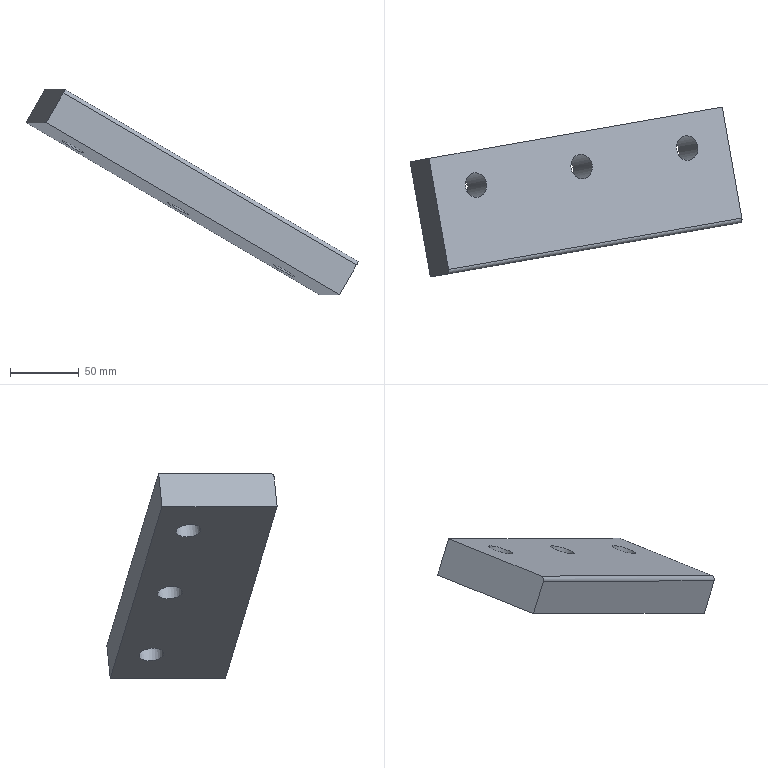Part | NX | features solid 2 | 1 solid | 10 faces | box 241.333 x 123.736 x 149.249 mm | volume 573142 mm3 | plane 6 | cylinder 4 | commonest cylinder face diameters 18 x3 6 x1
STEP:
#1=CARTESIAN_POINT('',(990.848,746.001,-183.512));
#2=VERTEX_POINT('',#1);
#3=CARTESIAN_POINT('',(777.631,708.405,-58.512));
#4=VERTEX_POINT('',#3);
#5=CARTESIAN_POINT('',(990.848,746.001,-183.512));
#6=DIRECTION('',(-0.8529,-0.1504,0.5));
#7=VECTOR('',#6,1000.);
#8=LINE('',#5,#7);
#9=EDGE_CURVE('',#2,#4,#8,.T.);
#10=ORIENTED_EDGE('',*,*,#9,.T.);
#11=CARTESIAN_POINT('',(791.418,710.836,-34.264));
#12=VERTEX_POINT('',#11);
#13=CARTESIAN_POINT('',(791.418,710.836,-34.264));
#14=DIRECTION('',(-0.4924,-0.08682,-0.866));
#15=VECTOR('',#14,1000.);
#16=LINE('',#13,#15);
#17=EDGE_CURVE('',#12,#4,#16,.T.);
#18=ORIENTED_EDGE('',*,*,#17,.F.);
#19=CARTESIAN_POINT('',(1004.635,748.432,-159.264));
#20=VERTEX_POINT('',#19);
#21=CARTESIAN_POINT('',(1004.635,748.432,-159.264));
#22=DIRECTION('',(-0.8529,-0.1504,0.5));
#23=VECTOR('',#22,1000.);
#24=LINE('',#21,#23);
#25=EDGE_CURVE('',#20,#12,#24,.T.);
#26=ORIENTED_EDGE('',*,*,#25,.F.);
#27=CARTESIAN_POINT('',(1004.635,748.432,-159.264));
#28=DIRECTION('',(-0.4924,-0.08682,-0.866));
#29=VECTOR('',#28,1000.);
#30=LINE('',#27,#29);
#31=EDGE_CURVE('',#20,#2,#30,.T.);
#32=ORIENTED_EDGE('',*,*,#31,.T.);
#33=EDGE_LOOP('',(#10,#18,#26,#32));
#34=FACE_BOUND('',#33,.T.);
#35=CARTESIAN_POINT('',(1004.635,748.432,-159.264));
#36=DIRECTION('',(-0.1736,0.9848,0.));
#37=DIRECTION('',(0.8529,0.1504,-0.5));
#38=AXIS2_PLACEMENT_3D('',#35,#36,#37);
#39=PLANE('',#38);
#40=ADVANCED_FACE('',(#34),#39,.T.);
#41=CARTESIAN_POINT('',(805.657,630.082,-34.264));
#42=VERTEX_POINT('',#41);
#43=CARTESIAN_POINT('',(792.807,702.957,-34.264));
#44=DIRECTION('',(0.1736,-0.9848,0.));
#45=VECTOR('',#44,1000.);
#46=LINE('',#43,#45);
#47=EDGE_CURVE('',#12,#42,#46,.T.);
#48=ORIENTED_EDGE('',*,*,#47,.F.);
#49=ORIENTED_EDGE('',*,*,#17,.T.);
#50=CARTESIAN_POINT('',(792.391,624.696,-58.512));
#51=VERTEX_POINT('',#50);
#52=CARTESIAN_POINT('',(779.02,700.526,-58.512));
#53=DIRECTION('',(0.1736,-0.9848,0.));
#54=VECTOR('',#53,1000.);
#55=LINE('',#52,#54);
#56=EDGE_CURVE('',#4,#51,#55,.T.);
#57=ORIENTED_EDGE('',*,*,#56,.T.);
#58=CARTESIAN_POINT('',(804.701,626.867,-36.862));
#59=VERTEX_POINT('',#58);
#60=CARTESIAN_POINT('',(806.178,627.127,-34.264));
#61=DIRECTION('',(-0.4924,-0.08682,-0.866));
#62=VECTOR('',#61,1000.);
#63=LINE('',#60,#62);
#64=EDGE_CURVE('',#59,#51,#63,.T.);
#65=ORIENTED_EDGE('',*,*,#64,.F.);
#66=CARTESIAN_POINT('',(804.18,629.821,-36.862));
#67=DIRECTION('',(0.8529,0.1504,-0.5));
#68=DIRECTION('',(0.4924,0.08682,0.866));
#69=AXIS2_PLACEMENT_3D('',#66,#67,#68);
#70=CIRCLE('',#69,3.);
#71=EDGE_CURVE('',#42,#59,#70,.T.);
#72=ORIENTED_EDGE('',*,*,#71,.F.);
#73=EDGE_LOOP('',(#48,#49,#57,#65,#72));
#74=FACE_BOUND('',#73,.T.);
#75=CARTESIAN_POINT('',(792.807,702.957,-34.264));
#76=DIRECTION('',(-0.8529,-0.1504,0.5));
#77=DIRECTION('',(0.4924,0.08682,0.866));
#78=AXIS2_PLACEMENT_3D('',#75,#76,#77);
#79=PLANE('',#78);
#80=ADVANCED_FACE('',(#74),#79,.T.);
#81=ORIENTED_EDGE('',*,*,#64,.T.);
#82=CARTESIAN_POINT('',(1005.608,662.292,-183.512));
#83=VERTEX_POINT('',#82);
#84=CARTESIAN_POINT('',(1005.608,662.292,-183.512));
#85=DIRECTION('',(0.8529,0.1504,-0.5));
#86=VECTOR('',#85,1000.);
#87=LINE('',#84,#86);
#88=EDGE_CURVE('',#51,#83,#87,.T.);
#89=ORIENTED_EDGE('',*,*,#88,.T.);
#90=CARTESIAN_POINT('',(1017.918,664.463,-161.862));
#91=VERTEX_POINT('',#90);
#92=CARTESIAN_POINT('',(1019.396,664.723,-159.264));
#93=DIRECTION('',(-0.4924,-0.08682,-0.866));
#94=VECTOR('',#93,1000.);
#95=LINE('',#92,#94);
#96=EDGE_CURVE('',#91,#83,#95,.T.);
#97=ORIENTED_EDGE('',*,*,#96,.F.);
#98=CARTESIAN_POINT('',(804.701,626.867,-36.862));
#99=DIRECTION('',(0.8529,0.1504,-0.5));
#100=VECTOR('',#99,1000.);
#101=LINE('',#98,#100);
#102=EDGE_CURVE('',#59,#91,#101,.T.);
#103=ORIENTED_EDGE('',*,*,#102,.F.);
#104=EDGE_LOOP('',(#81,#89,#97,#103));
#105=FACE_BOUND('',#104,.T.);
#106=CARTESIAN_POINT('',(806.178,627.127,-34.264));
#107=DIRECTION('',(0.1736,-0.9848,0.));
#108=DIRECTION('',(0.4924,0.08682,0.866));
#109=AXIS2_PLACEMENT_3D('',#106,#107,#108);
#110=PLANE('',#109);
#111=ADVANCED_FACE('',(#105),#110,.T.);
#112=ORIENTED_EDGE('',*,*,#96,.T.);
#113=CARTESIAN_POINT('',(992.237,738.122,-183.512));
#114=DIRECTION('',(-0.1736,0.9848,0.));
#115=VECTOR('',#114,1000.);
#116=LINE('',#113,#115);
#117=EDGE_CURVE('',#83,#2,#116,.T.);
#118=ORIENTED_EDGE('',*,*,#117,.T.);
#119=ORIENTED_EDGE('',*,*,#31,.F.);
#120=CARTESIAN_POINT('',(1018.875,667.677,-159.264));
#121=VERTEX_POINT('',#120);
#122=CARTESIAN_POINT('',(1018.527,669.647,-159.264));
#123=DIRECTION('',(-0.1736,0.9848,0.));
#124=VECTOR('',#123,1000.);
#125=LINE('',#122,#124);
#126=EDGE_CURVE('',#121,#20,#125,.T.);
#127=ORIENTED_EDGE('',*,*,#126,.F.);
#128=CARTESIAN_POINT('',(1017.397,667.417,-161.862));
#129=DIRECTION('',(-0.8529,-0.1504,0.5));
#130=DIRECTION('',(0.1736,-0.9848,0.));
#131=AXIS2_PLACEMENT_3D('',#128,#129,#130);
#132=CIRCLE('',#131,3.);
#133=EDGE_CURVE('',#91,#121,#132,.T.);
#134=ORIENTED_EDGE('',*,*,#133,.F.);
#135=EDGE_LOOP('',(#112,#118,#119,#127,#134));
#136=FACE_BOUND('',#135,.T.);
#137=CARTESIAN_POINT('',(1018.527,669.647,-159.264));
#138=DIRECTION('',(0.8529,0.1504,-0.5));
#139=DIRECTION('',(0.1736,-0.9848,0.));
#140=AXIS2_PLACEMENT_3D('',#137,#138,#139);
#141=PLANE('',#140);
#142=ADVANCED_FACE('',(#136),#141,.T.);
#143=CARTESIAN_POINT('',(894.692,703.66,-92.264));
#144=VERTEX_POINT('',#143);
#145=CARTESIAN_POINT('',(902.368,705.014,-96.764));
#146=DIRECTION('',(0.4924,0.08682,0.866));
#147=DIRECTION('',(-0.8529,-0.1504,0.5));
#148=AXIS2_PLACEMENT_3D('',#145,#146,#147);
#149=CIRCLE('',#148,9.);
#150=EDGE_CURVE('',#144,#144,#149,.T.);
#151=ORIENTED_EDGE('',*,*,#150,.F.);
#152=EDGE_LOOP('',(#151));
#153=FACE_BOUND('',#152,.T.);
#154=CARTESIAN_POINT('',(986.802,719.902,-146.264));
#155=VERTEX_POINT('',#154);
#156=CARTESIAN_POINT('',(979.126,718.548,-141.764));
#157=DIRECTION('',(-0.4924,-0.08682,-0.866));
#158=DIRECTION('',(0.8529,0.1504,-0.5));
#159=AXIS2_PLACEMENT_3D('',#156,#157,#158);
#160=CIRCLE('',#159,9.);
#161=EDGE_CURVE('',#155,#155,#160,.T.);
#162=ORIENTED_EDGE('',*,*,#161,.T.);
#163=EDGE_LOOP('',(#162));
#164=FACE_BOUND('',#163,.T.);
#165=CARTESIAN_POINT('',(817.934,690.126,-47.264));
#166=VERTEX_POINT('',#165);
#167=CARTESIAN_POINT('',(825.61,691.479,-51.764));
#168=DIRECTION('',(0.4924,0.08682,0.866));
#169=DIRECTION('',(-0.8529,-0.1504,0.5));
#170=AXIS2_PLACEMENT_3D('',#167,#168,#169);
#171=CIRCLE('',#170,9.);
#172=EDGE_CURVE('',#166,#166,#171,.T.);
#173=ORIENTED_EDGE('',*,*,#172,.F.);
#174=EDGE_LOOP('',(#173));
#175=FACE_BOUND('',#174,.T.);
#176=ORIENTED_EDGE('',*,*,#126,.T.);
#177=ORIENTED_EDGE('',*,*,#25,.T.);
#178=ORIENTED_EDGE('',*,*,#47,.T.);
#179=CARTESIAN_POINT('',(1018.875,667.677,-159.264));
#180=DIRECTION('',(0.8529,0.1504,-0.5));
#181=VECTOR('',#180,1000.);
#182=LINE('',#179,#181);
#183=EDGE_CURVE('',#121,#42,#182,.F.);
#184=ORIENTED_EDGE('',*,*,#183,.F.);
#185=EDGE_LOOP('',(#176,#177,#178,#184));
#186=FACE_BOUND('',#185,.T.);
#187=CARTESIAN_POINT('',(1006.025,740.553,-159.264));
#188=DIRECTION('',(0.4924,0.08682,0.866));
#189=DIRECTION('',(0.8529,0.1504,-0.5));
#190=AXIS2_PLACEMENT_3D('',#187,#188,#189);
#191=PLANE('',#190);
#192=ADVANCED_FACE('',(#153,#164,#175,#186),#191,.T.);
#193=CARTESIAN_POINT('',(881.229,699.907,-116.564));
#194=VERTEX_POINT('',#193);
#195=CARTESIAN_POINT('',(888.581,702.582,-121.012));
#196=DIRECTION('',(0.4924,0.08682,0.866));
#197=DIRECTION('',(-0.8169,-0.2973,0.4943));
#198=AXIS2_PLACEMENT_3D('',#195,#196,#197);
#199=CIRCLE('',#198,9.);
#200=EDGE_CURVE('',#194,#194,#199,.T.);
#201=ORIENTED_EDGE('',*,*,#200,.T.);
#202=EDGE_LOOP('',(#201));
#203=FACE_BOUND('',#202,.T.);
#204=CARTESIAN_POINT('',(957.987,713.441,-161.564));
#205=VERTEX_POINT('',#204);
#206=CARTESIAN_POINT('',(965.339,716.117,-166.012));
#207=DIRECTION('',(0.4924,0.08682,0.866));
#208=DIRECTION('',(-0.8169,-0.2973,0.4943));
#209=AXIS2_PLACEMENT_3D('',#206,#207,#208);
#210=CIRCLE('',#209,9.);
#211=EDGE_CURVE('',#205,#205,#210,.F.);
#212=ORIENTED_EDGE('',*,*,#211,.F.);
#213=EDGE_LOOP('',(#212));
#214=FACE_BOUND('',#213,.T.);
#215=CARTESIAN_POINT('',(804.471,686.372,-71.564));
#216=VERTEX_POINT('',#215);
#217=CARTESIAN_POINT('',(811.823,689.048,-76.012));
#218=DIRECTION('',(0.4924,0.08682,0.866));
#219=DIRECTION('',(-0.8169,-0.2973,0.4943));
#220=AXIS2_PLACEMENT_3D('',#217,#218,#219);
#221=CIRCLE('',#220,9.);
#222=EDGE_CURVE('',#216,#216,#221,.T.);
#223=ORIENTED_EDGE('',*,*,#222,.T.);
#224=EDGE_LOOP('',(#223));
#225=FACE_BOUND('',#224,.T.);
#226=ORIENTED_EDGE('',*,*,#9,.F.);
#227=ORIENTED_EDGE('',*,*,#117,.F.);
#228=ORIENTED_EDGE('',*,*,#88,.F.);
#229=ORIENTED_EDGE('',*,*,#56,.F.);
#230=EDGE_LOOP('',(#226,#227,#228,#229));
#231=FACE_BOUND('',#230,.T.);
#232=CARTESIAN_POINT('',(992.237,738.122,-183.512));
#233=DIRECTION('',(0.4924,0.08682,0.866));
#234=DIRECTION('',(0.8529,0.1504,-0.5));
#235=AXIS2_PLACEMENT_3D('',#232,#233,#234);
#236=PLANE('',#235);
#237=ADVANCED_FACE('',(#203,#214,#225,#231),#236,.F.);
#238=ORIENTED_EDGE('',*,*,#71,.T.);
#239=ORIENTED_EDGE('',*,*,#102,.T.);
#240=ORIENTED_EDGE('',*,*,#133,.T.);
#241=ORIENTED_EDGE('',*,*,#183,.T.);
#242=EDGE_LOOP('',(#238,#239,#240,#241));
#243=FACE_BOUND('',#242,.T.);
#244=CARTESIAN_POINT('',(804.18,629.821,-36.862));
#245=DIRECTION('',(0.8529,0.1504,-0.5));
#246=DIRECTION('',(-0.4924,-0.08682,-0.866));
#247=AXIS2_PLACEMENT_3D('',#244,#245,#246);
#248=CYLINDRICAL_SURFACE('',#247,3.);
#249=ADVANCED_FACE('',(#243),#248,.T.);
#250=ORIENTED_EDGE('',*,*,#222,.F.);
#251=EDGE_LOOP('',(#250));
#252=FACE_BOUND('',#251,.T.);
#253=ORIENTED_EDGE('',*,*,#172,.T.);
#254=EDGE_LOOP('',(#253));
#255=FACE_BOUND('',#254,.T.);
#256=CARTESIAN_POINT('',(825.61,691.479,-51.764));
#257=DIRECTION('',(-0.4924,-0.08682,-0.866));
#258=DIRECTION('',(-0.8529,-0.1504,0.5));
#259=AXIS2_PLACEMENT_3D('',#256,#257,#258);
#260=CYLINDRICAL_SURFACE('',#259,9.);
#261=ADVANCED_FACE('',(#252,#255),#260,.F.);
#262=ORIENTED_EDGE('',*,*,#211,.T.);
#263=EDGE_LOOP('',(#262));
#264=FACE_BOUND('',#263,.T.);
#265=ORIENTED_EDGE('',*,*,#161,.F.);
#266=EDGE_LOOP('',(#265));
#267=FACE_BOUND('',#266,.T.);
#268=CARTESIAN_POINT('',(979.126,718.548,-141.764));
#269=DIRECTION('',(-0.4924,-0.08682,-0.866));
#270=DIRECTION('',(0.8529,0.1504,-0.5));
#271=AXIS2_PLACEMENT_3D('',#268,#269,#270);
#272=CYLINDRICAL_SURFACE('',#271,9.);
#273=ADVANCED_FACE('',(#264,#267),#272,.F.);
#274=ORIENTED_EDGE('',*,*,#200,.F.);
#275=EDGE_LOOP('',(#274));
#276=FACE_BOUND('',#275,.T.);
#277=ORIENTED_EDGE('',*,*,#150,.T.);
#278=EDGE_LOOP('',(#277));
#279=FACE_BOUND('',#278,.T.);
#280=CARTESIAN_POINT('',(902.368,705.014,-96.764));
#281=DIRECTION('',(-0.4924,-0.08682,-0.866));
#282=DIRECTION('',(-0.8529,-0.1504,0.5));
#283=AXIS2_PLACEMENT_3D('',#280,#281,#282);
#284=CYLINDRICAL_SURFACE('',#283,9.);
#285=ADVANCED_FACE('',(#276,#279),#284,.F.);
#286=CLOSED_SHELL('',(#40,#80,#111,#142,#192,#237,#249,#261,#273,#285));
#287=MANIFOLD_SOLID_BREP('',#286);
#288=(LENGTH_UNIT()NAMED_UNIT(*)SI_UNIT(.MILLI.,.METRE.));
#289=UNCERTAINTY_MEASURE_WITH_UNIT(LENGTH_MEASURE(0.00001),#288,'','');
#290=(NAMED_UNIT(*)PLANE_ANGLE_UNIT()SI_UNIT($,.RADIAN.));
#291=(NAMED_UNIT(*)SI_UNIT($,.STERADIAN.)SOLID_ANGLE_UNIT());
#292=(GEOMETRIC_REPRESENTATION_CONTEXT(3)GLOBAL_UNCERTAINTY_ASSIGNED_CONTEXT((#289))GLOBAL_UNIT_ASSIGNED_CONTEXT((#288,#290,#291))REPRESENTATION_CONTEXT('',''));
#293=ADVANCED_BREP_SHAPE_REPRESENTATION('',(#287),#292);